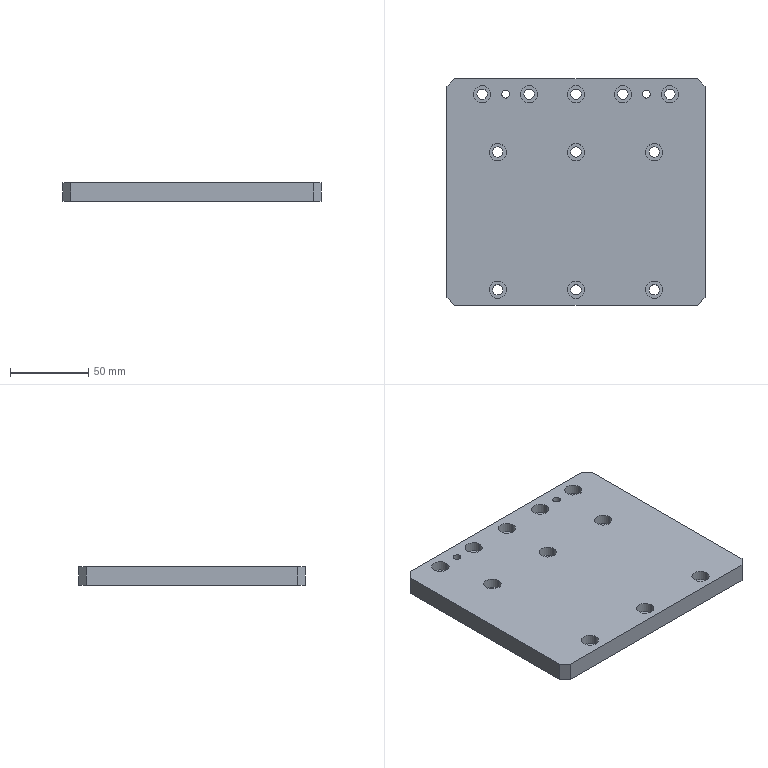Part | NX | features BREP 1 | 1 solid | 69 faces | box 165 x 145 x 12 mm | volume 277231 mm3 | cylinder 48 | plane 21 | commonest cylinder face diameters 6.6 x22 11 x22 5 x4